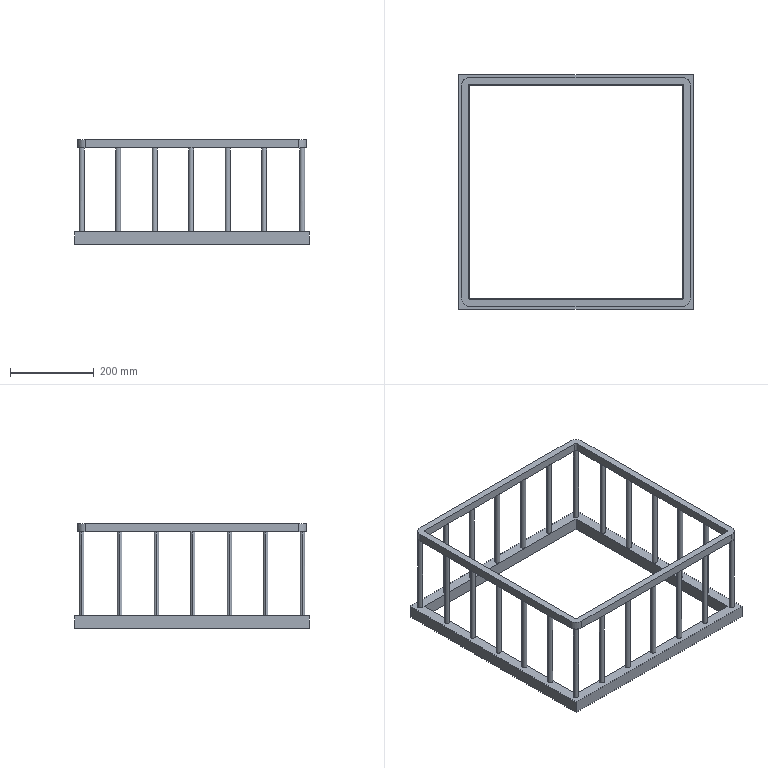Part | SolidWorks | features ICE 2, Extrusion 1 | 1 solid | 80 faces | box 560 x 560 x 250 mm | volume 2819829 mm3 | cylinder 56 | plane 24 | commonest cylinder face diameters 12 x48 10 x4 40 x4